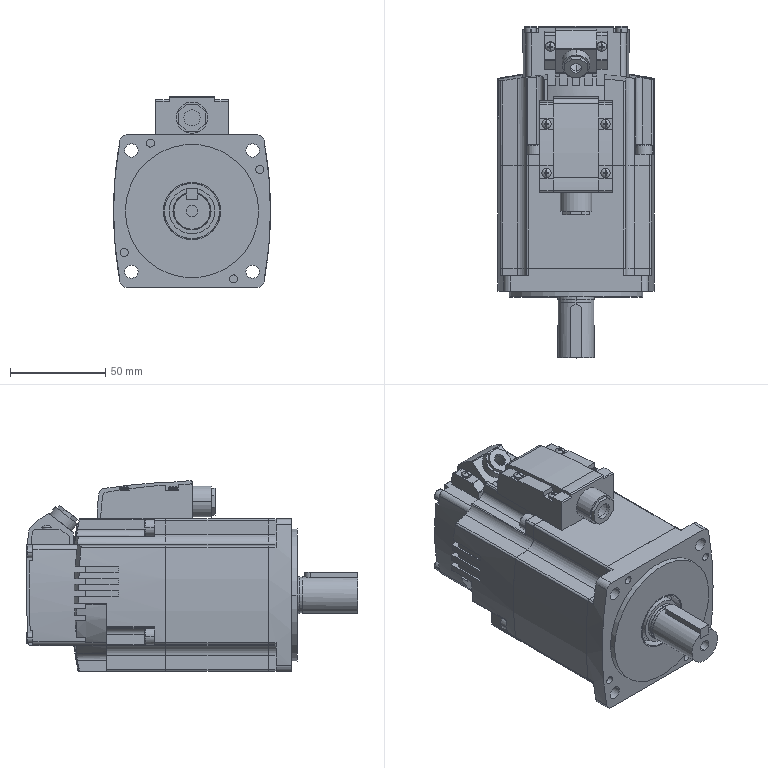Part | SolidWorks | features MBimport 1 | 8 solids | 845 faces | box 82.337 x 174.253 x 100 mm | volume 739661 mm3 | plane 527 | cylinder 244 | torus 52 | sphere 22 | commonest cylinder face diameters 2 x26 7 x19 1.2 x17 5 x12 10.6 x12 8.72 x10